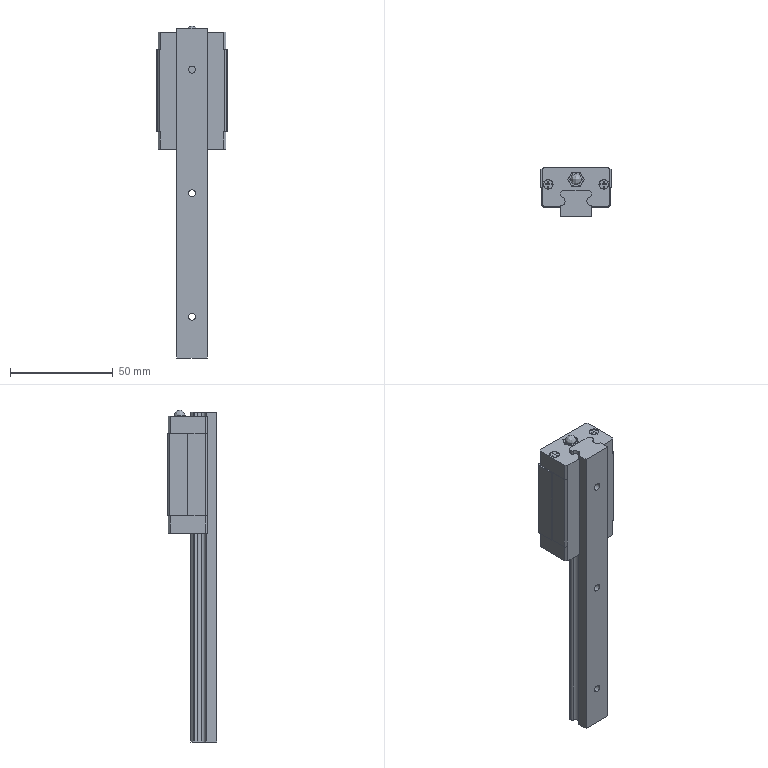Part | SolidWorks | 2 solids | 206 faces | box 34 x 24 x 161.094 mm | volume 57035 mm3 | plane 119 | cylinder 70 | cone 16 | spline 1 | commonest cylinder face diameters 3.08 x20 4.4 x14 3.242 x8 4.8 x8 3.5 x6 6 x6